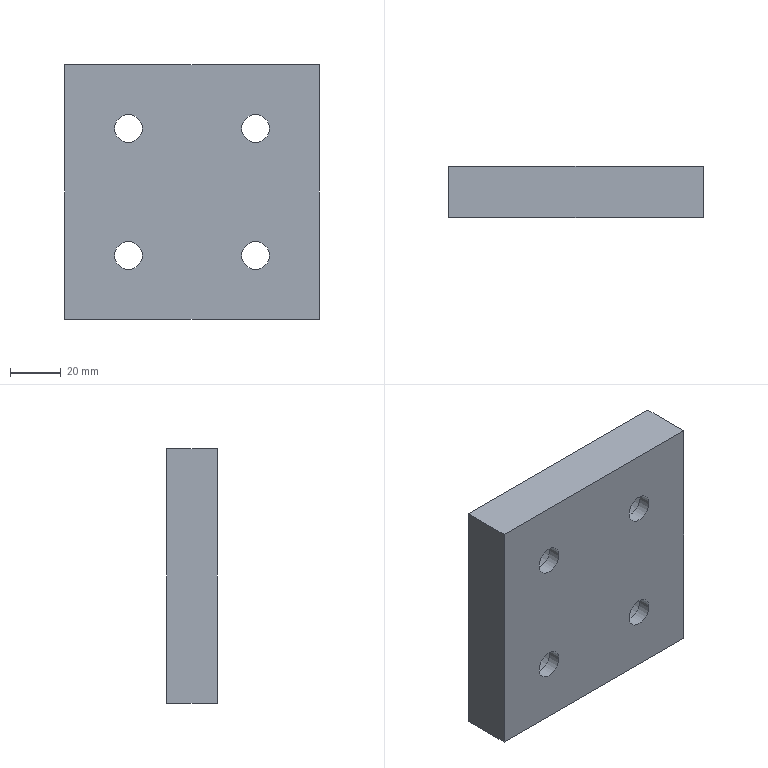Part | NX | features solid 2 | 1 solid | 18 faces | box 100 x 20 x 100 mm | volume 183668 mm3 | plane 10 | cylinder 8 | commonest cylinder face diameters 11 x4 17.5 x4
STEP:
#1=CARTESIAN_POINT('',(-1100.,530.,-135.));
#2=VERTEX_POINT('',#1);
#3=CARTESIAN_POINT('',(-1100.,510.,-135.));
#4=VERTEX_POINT('',#3);
#5=CARTESIAN_POINT('',(-1100.,520.,-135.));
#6=DIRECTION('',(0.,-1.,0.));
#7=VECTOR('',#6,1000.);
#8=LINE('',#5,#7);
#9=EDGE_CURVE('',#2,#4,#8,.T.);
#10=ORIENTED_EDGE('',*,*,#9,.F.);
#11=CARTESIAN_POINT('',(-1000.,530.,-135.));
#12=VERTEX_POINT('',#11);
#13=CARTESIAN_POINT('',(-1050.,530.,-135.));
#14=DIRECTION('',(-1.,0.,0.));
#15=VECTOR('',#14,1000.);
#16=LINE('',#13,#15);
#17=EDGE_CURVE('',#12,#2,#16,.T.);
#18=ORIENTED_EDGE('',*,*,#17,.F.);
#19=CARTESIAN_POINT('',(-1000.,510.,-135.));
#20=VERTEX_POINT('',#19);
#21=CARTESIAN_POINT('',(-1000.,520.,-135.));
#22=DIRECTION('',(0.,1.,0.));
#23=VECTOR('',#22,1000.);
#24=LINE('',#21,#23);
#25=EDGE_CURVE('',#20,#12,#24,.T.);
#26=ORIENTED_EDGE('',*,*,#25,.F.);
#27=CARTESIAN_POINT('',(-1050.,510.,-135.));
#28=DIRECTION('',(1.,0.,0.));
#29=VECTOR('',#28,1000.);
#30=LINE('',#27,#29);
#31=EDGE_CURVE('',#4,#20,#30,.T.);
#32=ORIENTED_EDGE('',*,*,#31,.F.);
#33=EDGE_LOOP('',(#10,#18,#26,#32));
#34=FACE_BOUND('',#33,.T.);
#35=CARTESIAN_POINT('',(-1050.,520.,-135.));
#36=DIRECTION('',(0.,0.,-1.));
#37=DIRECTION('',(0.,1.,0.));
#38=AXIS2_PLACEMENT_3D('',#35,#36,#37);
#39=PLANE('',#38);
#40=ADVANCED_FACE('',(#34),#39,.T.);
#41=CARTESIAN_POINT('',(-1100.,530.,-35.));
#42=VERTEX_POINT('',#41);
#43=CARTESIAN_POINT('',(-1100.,530.,-35.));
#44=DIRECTION('',(0.,0.,-1.));
#45=VECTOR('',#44,1000.);
#46=LINE('',#43,#45);
#47=EDGE_CURVE('',#42,#2,#46,.T.);
#48=ORIENTED_EDGE('',*,*,#47,.T.);
#49=ORIENTED_EDGE('',*,*,#9,.T.);
#50=CARTESIAN_POINT('',(-1100.,510.,-35.));
#51=VERTEX_POINT('',#50);
#52=CARTESIAN_POINT('',(-1100.,510.,-35.));
#53=DIRECTION('',(0.,0.,-1.));
#54=VECTOR('',#53,1000.);
#55=LINE('',#52,#54);
#56=EDGE_CURVE('',#51,#4,#55,.T.);
#57=ORIENTED_EDGE('',*,*,#56,.F.);
#58=CARTESIAN_POINT('',(-1100.,520.,-35.));
#59=DIRECTION('',(0.,1.,0.));
#60=VECTOR('',#59,1000.);
#61=LINE('',#58,#60);
#62=EDGE_CURVE('',#51,#42,#61,.T.);
#63=ORIENTED_EDGE('',*,*,#62,.T.);
#64=EDGE_LOOP('',(#48,#49,#57,#63));
#65=FACE_BOUND('',#64,.T.);
#66=CARTESIAN_POINT('',(-1100.,520.,-35.));
#67=DIRECTION('',(-1.,0.,0.));
#68=DIRECTION('',(0.,0.,1.));
#69=AXIS2_PLACEMENT_3D('',#66,#67,#68);
#70=PLANE('',#69);
#71=ADVANCED_FACE('',(#65),#70,.T.);
#72=CARTESIAN_POINT('',(-1025.,510.,-54.5));
#73=VERTEX_POINT('',#72);
#74=CARTESIAN_POINT('',(-1025.,510.,-60.));
#75=DIRECTION('',(0.,1.,0.));
#76=DIRECTION('',(0.,0.,1.));
#77=AXIS2_PLACEMENT_3D('',#74,#75,#76);
#78=CIRCLE('',#77,5.5);
#79=EDGE_CURVE('',#73,#73,#78,.T.);
#80=ORIENTED_EDGE('',*,*,#79,.T.);
#81=EDGE_LOOP('',(#80));
#82=FACE_BOUND('',#81,.T.);
#83=CARTESIAN_POINT('',(-1025.,510.,-104.5));
#84=VERTEX_POINT('',#83);
#85=CARTESIAN_POINT('',(-1025.,510.,-110.));
#86=DIRECTION('',(0.,1.,0.));
#87=DIRECTION('',(0.,0.,1.));
#88=AXIS2_PLACEMENT_3D('',#85,#86,#87);
#89=CIRCLE('',#88,5.5);
#90=EDGE_CURVE('',#84,#84,#89,.T.);
#91=ORIENTED_EDGE('',*,*,#90,.T.);
#92=EDGE_LOOP('',(#91));
#93=FACE_BOUND('',#92,.T.);
#94=CARTESIAN_POINT('',(-1075.,510.,-54.5));
#95=VERTEX_POINT('',#94);
#96=CARTESIAN_POINT('',(-1075.,510.,-60.));
#97=DIRECTION('',(0.,1.,0.));
#98=DIRECTION('',(0.,0.,1.));
#99=AXIS2_PLACEMENT_3D('',#96,#97,#98);
#100=CIRCLE('',#99,5.5);
#101=EDGE_CURVE('',#95,#95,#100,.T.);
#102=ORIENTED_EDGE('',*,*,#101,.T.);
#103=EDGE_LOOP('',(#102));
#104=FACE_BOUND('',#103,.T.);
#105=CARTESIAN_POINT('',(-1075.,510.,-104.5));
#106=VERTEX_POINT('',#105);
#107=CARTESIAN_POINT('',(-1075.,510.,-110.));
#108=DIRECTION('',(0.,1.,0.));
#109=DIRECTION('',(0.,0.,1.));
#110=AXIS2_PLACEMENT_3D('',#107,#108,#109);
#111=CIRCLE('',#110,5.5);
#112=EDGE_CURVE('',#106,#106,#111,.T.);
#113=ORIENTED_EDGE('',*,*,#112,.T.);
#114=EDGE_LOOP('',(#113));
#115=FACE_BOUND('',#114,.T.);
#116=ORIENTED_EDGE('',*,*,#56,.T.);
#117=ORIENTED_EDGE('',*,*,#31,.T.);
#118=CARTESIAN_POINT('',(-1000.,510.,-35.));
#119=VERTEX_POINT('',#118);
#120=CARTESIAN_POINT('',(-1000.,510.,-35.));
#121=DIRECTION('',(0.,0.,-1.));
#122=VECTOR('',#121,1000.);
#123=LINE('',#120,#122);
#124=EDGE_CURVE('',#119,#20,#123,.T.);
#125=ORIENTED_EDGE('',*,*,#124,.F.);
#126=CARTESIAN_POINT('',(-1050.,510.,-35.));
#127=DIRECTION('',(-1.,0.,0.));
#128=VECTOR('',#127,1000.);
#129=LINE('',#126,#128);
#130=EDGE_CURVE('',#119,#51,#129,.T.);
#131=ORIENTED_EDGE('',*,*,#130,.T.);
#132=EDGE_LOOP('',(#116,#117,#125,#131));
#133=FACE_BOUND('',#132,.T.);
#134=CARTESIAN_POINT('',(-1050.,510.,-35.));
#135=DIRECTION('',(0.,-1.,0.));
#136=DIRECTION('',(0.,0.,-1.));
#137=AXIS2_PLACEMENT_3D('',#134,#135,#136);
#138=PLANE('',#137);
#139=ADVANCED_FACE('',(#82,#93,#104,#115,#133),#138,.T.);
#140=ORIENTED_EDGE('',*,*,#124,.T.);
#141=ORIENTED_EDGE('',*,*,#25,.T.);
#142=CARTESIAN_POINT('',(-1000.,530.,-35.));
#143=VERTEX_POINT('',#142);
#144=CARTESIAN_POINT('',(-1000.,530.,-35.));
#145=DIRECTION('',(0.,0.,-1.));
#146=VECTOR('',#145,1000.);
#147=LINE('',#144,#146);
#148=EDGE_CURVE('',#143,#12,#147,.T.);
#149=ORIENTED_EDGE('',*,*,#148,.F.);
#150=CARTESIAN_POINT('',(-1000.,520.,-35.));
#151=DIRECTION('',(0.,-1.,0.));
#152=VECTOR('',#151,1000.);
#153=LINE('',#150,#152);
#154=EDGE_CURVE('',#143,#119,#153,.T.);
#155=ORIENTED_EDGE('',*,*,#154,.T.);
#156=EDGE_LOOP('',(#140,#141,#149,#155));
#157=FACE_BOUND('',#156,.T.);
#158=CARTESIAN_POINT('',(-1000.,520.,-35.));
#159=DIRECTION('',(1.,0.,0.));
#160=DIRECTION('',(0.,0.,-1.));
#161=AXIS2_PLACEMENT_3D('',#158,#159,#160);
#162=PLANE('',#161);
#163=ADVANCED_FACE('',(#157),#162,.T.);
#164=CARTESIAN_POINT('',(-1050.,530.,-35.));
#165=DIRECTION('',(1.,0.,0.));
#166=VECTOR('',#165,1000.);
#167=LINE('',#164,#166);
#168=EDGE_CURVE('',#42,#143,#167,.T.);
#169=ORIENTED_EDGE('',*,*,#168,.F.);
#170=ORIENTED_EDGE('',*,*,#62,.F.);
#171=ORIENTED_EDGE('',*,*,#130,.F.);
#172=ORIENTED_EDGE('',*,*,#154,.F.);
#173=EDGE_LOOP('',(#169,#170,#171,#172));
#174=FACE_BOUND('',#173,.T.);
#175=CARTESIAN_POINT('',(-1050.,520.,-35.));
#176=DIRECTION('',(0.,0.,1.));
#177=DIRECTION('',(0.,-1.,0.));
#178=AXIS2_PLACEMENT_3D('',#175,#176,#177);
#179=PLANE('',#178);
#180=ADVANCED_FACE('',(#174),#179,.T.);
#181=CARTESIAN_POINT('',(-1025.,530.,-68.75));
#182=VERTEX_POINT('',#181);
#183=CARTESIAN_POINT('',(-1025.,530.,-60.));
#184=DIRECTION('',(0.,-1.,0.));
#185=DIRECTION('',(0.,0.,-1.));
#186=AXIS2_PLACEMENT_3D('',#183,#184,#185);
#187=CIRCLE('',#186,8.75);
#188=EDGE_CURVE('',#182,#182,#187,.T.);
#189=ORIENTED_EDGE('',*,*,#188,.T.);
#190=EDGE_LOOP('',(#189));
#191=FACE_BOUND('',#190,.T.);
#192=CARTESIAN_POINT('',(-1025.,530.,-118.75));
#193=VERTEX_POINT('',#192);
#194=CARTESIAN_POINT('',(-1025.,530.,-110.));
#195=DIRECTION('',(0.,-1.,0.));
#196=DIRECTION('',(0.,0.,-1.));
#197=AXIS2_PLACEMENT_3D('',#194,#195,#196);
#198=CIRCLE('',#197,8.75);
#199=EDGE_CURVE('',#193,#193,#198,.T.);
#200=ORIENTED_EDGE('',*,*,#199,.T.);
#201=EDGE_LOOP('',(#200));
#202=FACE_BOUND('',#201,.T.);
#203=CARTESIAN_POINT('',(-1075.,530.,-68.75));
#204=VERTEX_POINT('',#203);
#205=CARTESIAN_POINT('',(-1075.,530.,-60.));
#206=DIRECTION('',(0.,-1.,0.));
#207=DIRECTION('',(0.,0.,-1.));
#208=AXIS2_PLACEMENT_3D('',#205,#206,#207);
#209=CIRCLE('',#208,8.75);
#210=EDGE_CURVE('',#204,#204,#209,.T.);
#211=ORIENTED_EDGE('',*,*,#210,.T.);
#212=EDGE_LOOP('',(#211));
#213=FACE_BOUND('',#212,.T.);
#214=CARTESIAN_POINT('',(-1075.,530.,-118.75));
#215=VERTEX_POINT('',#214);
#216=CARTESIAN_POINT('',(-1075.,530.,-110.));
#217=DIRECTION('',(0.,-1.,0.));
#218=DIRECTION('',(0.,0.,-1.));
#219=AXIS2_PLACEMENT_3D('',#216,#217,#218);
#220=CIRCLE('',#219,8.75);
#221=EDGE_CURVE('',#215,#215,#220,.T.);
#222=ORIENTED_EDGE('',*,*,#221,.T.);
#223=EDGE_LOOP('',(#222));
#224=FACE_BOUND('',#223,.T.);
#225=ORIENTED_EDGE('',*,*,#168,.T.);
#226=ORIENTED_EDGE('',*,*,#148,.T.);
#227=ORIENTED_EDGE('',*,*,#17,.T.);
#228=ORIENTED_EDGE('',*,*,#47,.F.);
#229=EDGE_LOOP('',(#225,#226,#227,#228));
#230=FACE_BOUND('',#229,.T.);
#231=CARTESIAN_POINT('',(-1050.,530.,-35.));
#232=DIRECTION('',(0.,1.,0.));
#233=DIRECTION('',(0.,0.,1.));
#234=AXIS2_PLACEMENT_3D('',#231,#232,#233);
#235=PLANE('',#234);
#236=ADVANCED_FACE('',(#191,#202,#213,#224,#230),#235,.T.);
#237=CARTESIAN_POINT('',(-1075.,515.,-115.5));
#238=VERTEX_POINT('',#237);
#239=CARTESIAN_POINT('',(-1075.,515.,-110.));
#240=DIRECTION('',(0.,-1.,0.));
#241=DIRECTION('',(0.,0.,-1.));
#242=AXIS2_PLACEMENT_3D('',#239,#240,#241);
#243=CIRCLE('',#242,5.5);
#244=EDGE_CURVE('',#238,#238,#243,.F.);
#245=ORIENTED_EDGE('',*,*,#244,.T.);
#246=EDGE_LOOP('',(#245));
#247=FACE_BOUND('',#246,.T.);
#248=ORIENTED_EDGE('',*,*,#112,.F.);
#249=EDGE_LOOP('',(#248));
#250=FACE_BOUND('',#249,.T.);
#251=CARTESIAN_POINT('',(-1075.,510.,-110.));
#252=DIRECTION('',(0.,1.,0.));
#253=DIRECTION('',(0.,0.,1.));
#254=AXIS2_PLACEMENT_3D('',#251,#252,#253);
#255=CYLINDRICAL_SURFACE('',#254,5.5);
#256=ADVANCED_FACE('',(#247,#250),#255,.F.);
#257=CARTESIAN_POINT('',(-1075.,515.,-101.25));
#258=VERTEX_POINT('',#257);
#259=CARTESIAN_POINT('',(-1075.,515.,-110.));
#260=DIRECTION('',(0.,1.,0.));
#261=DIRECTION('',(0.,0.,1.));
#262=AXIS2_PLACEMENT_3D('',#259,#260,#261);
#263=CIRCLE('',#262,8.75);
#264=EDGE_CURVE('',#258,#258,#263,.T.);
#265=ORIENTED_EDGE('',*,*,#264,.T.);
#266=EDGE_LOOP('',(#265));
#267=FACE_BOUND('',#266,.T.);
#268=ORIENTED_EDGE('',*,*,#244,.F.);
#269=EDGE_LOOP('',(#268));
#270=FACE_BOUND('',#269,.T.);
#271=CARTESIAN_POINT('',(-1075.,515.,-110.));
#272=DIRECTION('',(0.,-1.,0.));
#273=DIRECTION('',(0.,0.,-1.));
#274=AXIS2_PLACEMENT_3D('',#271,#272,#273);
#275=PLANE('',#274);
#276=ADVANCED_FACE('',(#267,#270),#275,.F.);
#277=ORIENTED_EDGE('',*,*,#221,.F.);
#278=EDGE_LOOP('',(#277));
#279=FACE_BOUND('',#278,.T.);
#280=ORIENTED_EDGE('',*,*,#264,.F.);
#281=EDGE_LOOP('',(#280));
#282=FACE_BOUND('',#281,.T.);
#283=CARTESIAN_POINT('',(-1075.,515.,-110.));
#284=DIRECTION('',(0.,1.,0.));
#285=DIRECTION('',(0.,0.,1.));
#286=AXIS2_PLACEMENT_3D('',#283,#284,#285);
#287=CYLINDRICAL_SURFACE('',#286,8.75);
#288=ADVANCED_FACE('',(#279,#282),#287,.F.);
#289=CARTESIAN_POINT('',(-1075.,515.,-65.5));
#290=VERTEX_POINT('',#289);
#291=CARTESIAN_POINT('',(-1075.,515.,-60.));
#292=DIRECTION('',(0.,-1.,0.));
#293=DIRECTION('',(0.,0.,-1.));
#294=AXIS2_PLACEMENT_3D('',#291,#292,#293);
#295=CIRCLE('',#294,5.5);
#296=EDGE_CURVE('',#290,#290,#295,.F.);
#297=ORIENTED_EDGE('',*,*,#296,.T.);
#298=EDGE_LOOP('',(#297));
#299=FACE_BOUND('',#298,.T.);
#300=ORIENTED_EDGE('',*,*,#101,.F.);
#301=EDGE_LOOP('',(#300));
#302=FACE_BOUND('',#301,.T.);
#303=CARTESIAN_POINT('',(-1075.,510.,-60.));
#304=DIRECTION('',(0.,1.,0.));
#305=DIRECTION('',(0.,0.,1.));
#306=AXIS2_PLACEMENT_3D('',#303,#304,#305);
#307=CYLINDRICAL_SURFACE('',#306,5.5);
#308=ADVANCED_FACE('',(#299,#302),#307,.F.);
#309=CARTESIAN_POINT('',(-1075.,515.,-51.25));
#310=VERTEX_POINT('',#309);
#311=CARTESIAN_POINT('',(-1075.,515.,-60.));
#312=DIRECTION('',(0.,1.,0.));
#313=DIRECTION('',(0.,0.,1.));
#314=AXIS2_PLACEMENT_3D('',#311,#312,#313);
#315=CIRCLE('',#314,8.75);
#316=EDGE_CURVE('',#310,#310,#315,.T.);
#317=ORIENTED_EDGE('',*,*,#316,.T.);
#318=EDGE_LOOP('',(#317));
#319=FACE_BOUND('',#318,.T.);
#320=ORIENTED_EDGE('',*,*,#296,.F.);
#321=EDGE_LOOP('',(#320));
#322=FACE_BOUND('',#321,.T.);
#323=CARTESIAN_POINT('',(-1075.,515.,-60.));
#324=DIRECTION('',(0.,-1.,0.));
#325=DIRECTION('',(0.,0.,-1.));
#326=AXIS2_PLACEMENT_3D('',#323,#324,#325);
#327=PLANE('',#326);
#328=ADVANCED_FACE('',(#319,#322),#327,.F.);
#329=ORIENTED_EDGE('',*,*,#210,.F.);
#330=EDGE_LOOP('',(#329));
#331=FACE_BOUND('',#330,.T.);
#332=ORIENTED_EDGE('',*,*,#316,.F.);
#333=EDGE_LOOP('',(#332));
#334=FACE_BOUND('',#333,.T.);
#335=CARTESIAN_POINT('',(-1075.,515.,-60.));
#336=DIRECTION('',(0.,1.,0.));
#337=DIRECTION('',(0.,0.,1.));
#338=AXIS2_PLACEMENT_3D('',#335,#336,#337);
#339=CYLINDRICAL_SURFACE('',#338,8.75);
#340=ADVANCED_FACE('',(#331,#334),#339,.F.);
#341=CARTESIAN_POINT('',(-1025.,515.,-115.5));
#342=VERTEX_POINT('',#341);
#343=CARTESIAN_POINT('',(-1025.,515.,-110.));
#344=DIRECTION('',(0.,-1.,0.));
#345=DIRECTION('',(0.,0.,-1.));
#346=AXIS2_PLACEMENT_3D('',#343,#344,#345);
#347=CIRCLE('',#346,5.5);
#348=EDGE_CURVE('',#342,#342,#347,.F.);
#349=ORIENTED_EDGE('',*,*,#348,.T.);
#350=EDGE_LOOP('',(#349));
#351=FACE_BOUND('',#350,.T.);
#352=ORIENTED_EDGE('',*,*,#90,.F.);
#353=EDGE_LOOP('',(#352));
#354=FACE_BOUND('',#353,.T.);
#355=CARTESIAN_POINT('',(-1025.,510.,-110.));
#356=DIRECTION('',(0.,1.,0.));
#357=DIRECTION('',(0.,0.,1.));
#358=AXIS2_PLACEMENT_3D('',#355,#356,#357);
#359=CYLINDRICAL_SURFACE('',#358,5.5);
#360=ADVANCED_FACE('',(#351,#354),#359,.F.);
#361=CARTESIAN_POINT('',(-1025.,515.,-101.25));
#362=VERTEX_POINT('',#361);
#363=CARTESIAN_POINT('',(-1025.,515.,-110.));
#364=DIRECTION('',(0.,1.,0.));
#365=DIRECTION('',(0.,0.,1.));
#366=AXIS2_PLACEMENT_3D('',#363,#364,#365);
#367=CIRCLE('',#366,8.75);
#368=EDGE_CURVE('',#362,#362,#367,.T.);
#369=ORIENTED_EDGE('',*,*,#368,.T.);
#370=EDGE_LOOP('',(#369));
#371=FACE_BOUND('',#370,.T.);
#372=ORIENTED_EDGE('',*,*,#348,.F.);
#373=EDGE_LOOP('',(#372));
#374=FACE_BOUND('',#373,.T.);
#375=CARTESIAN_POINT('',(-1025.,515.,-110.));
#376=DIRECTION('',(0.,-1.,0.));
#377=DIRECTION('',(0.,0.,-1.));
#378=AXIS2_PLACEMENT_3D('',#375,#376,#377);
#379=PLANE('',#378);
#380=ADVANCED_FACE('',(#371,#374),#379,.F.);
#381=ORIENTED_EDGE('',*,*,#199,.F.);
#382=EDGE_LOOP('',(#381));
#383=FACE_BOUND('',#382,.T.);
#384=ORIENTED_EDGE('',*,*,#368,.F.);
#385=EDGE_LOOP('',(#384));
#386=FACE_BOUND('',#385,.T.);
#387=CARTESIAN_POINT('',(-1025.,515.,-110.));
#388=DIRECTION('',(0.,1.,0.));
#389=DIRECTION('',(0.,0.,1.));
#390=AXIS2_PLACEMENT_3D('',#387,#388,#389);
#391=CYLINDRICAL_SURFACE('',#390,8.75);
#392=ADVANCED_FACE('',(#383,#386),#391,.F.);
#393=CARTESIAN_POINT('',(-1025.,515.,-65.5));
#394=VERTEX_POINT('',#393);
#395=CARTESIAN_POINT('',(-1025.,515.,-60.));
#396=DIRECTION('',(0.,-1.,0.));
#397=DIRECTION('',(0.,0.,-1.));
#398=AXIS2_PLACEMENT_3D('',#395,#396,#397);
#399=CIRCLE('',#398,5.5);
#400=EDGE_CURVE('',#394,#394,#399,.F.);
#401=ORIENTED_EDGE('',*,*,#400,.T.);
#402=EDGE_LOOP('',(#401));
#403=FACE_BOUND('',#402,.T.);
#404=ORIENTED_EDGE('',*,*,#79,.F.);
#405=EDGE_LOOP('',(#404));
#406=FACE_BOUND('',#405,.T.);
#407=CARTESIAN_POINT('',(-1025.,510.,-60.));
#408=DIRECTION('',(0.,1.,0.));
#409=DIRECTION('',(0.,0.,1.));
#410=AXIS2_PLACEMENT_3D('',#407,#408,#409);
#411=CYLINDRICAL_SURFACE('',#410,5.5);
#412=ADVANCED_FACE('',(#403,#406),#411,.F.);
#413=CARTESIAN_POINT('',(-1025.,515.,-51.25));
#414=VERTEX_POINT('',#413);
#415=CARTESIAN_POINT('',(-1025.,515.,-60.));
#416=DIRECTION('',(0.,1.,0.));
#417=DIRECTION('',(0.,0.,1.));
#418=AXIS2_PLACEMENT_3D('',#415,#416,#417);
#419=CIRCLE('',#418,8.75);
#420=EDGE_CURVE('',#414,#414,#419,.T.);
#421=ORIENTED_EDGE('',*,*,#420,.T.);
#422=EDGE_LOOP('',(#421));
#423=FACE_BOUND('',#422,.T.);
#424=ORIENTED_EDGE('',*,*,#400,.F.);
#425=EDGE_LOOP('',(#424));
#426=FACE_BOUND('',#425,.T.);
#427=CARTESIAN_POINT('',(-1025.,515.,-60.));
#428=DIRECTION('',(0.,-1.,0.));
#429=DIRECTION('',(0.,0.,-1.));
#430=AXIS2_PLACEMENT_3D('',#427,#428,#429);
#431=PLANE('',#430);
#432=ADVANCED_FACE('',(#423,#426),#431,.F.);
#433=ORIENTED_EDGE('',*,*,#188,.F.);
#434=EDGE_LOOP('',(#433));
#435=FACE_BOUND('',#434,.T.);
#436=ORIENTED_EDGE('',*,*,#420,.F.);
#437=EDGE_LOOP('',(#436));
#438=FACE_BOUND('',#437,.T.);
#439=CARTESIAN_POINT('',(-1025.,515.,-60.));
#440=DIRECTION('',(0.,1.,0.));
#441=DIRECTION('',(0.,0.,1.));
#442=AXIS2_PLACEMENT_3D('',#439,#440,#441);
#443=CYLINDRICAL_SURFACE('',#442,8.75);
#444=ADVANCED_FACE('',(#435,#438),#443,.F.);
#445=CLOSED_SHELL('',(#40,#71,#139,#163,#180,#236,#256,#276,#288,#308,#328,#340,#360,#380,#392,#412,#432,#444));
#446=MANIFOLD_SOLID_BREP('',#445);
#447=(LENGTH_UNIT()NAMED_UNIT(*)SI_UNIT(.MILLI.,.METRE.));
#448=UNCERTAINTY_MEASURE_WITH_UNIT(LENGTH_MEASURE(0.00001),#447,'','');
#449=(NAMED_UNIT(*)PLANE_ANGLE_UNIT()SI_UNIT($,.RADIAN.));
#450=(NAMED_UNIT(*)SI_UNIT($,.STERADIAN.)SOLID_ANGLE_UNIT());
#451=(GEOMETRIC_REPRESENTATION_CONTEXT(3)GLOBAL_UNCERTAINTY_ASSIGNED_CONTEXT((#448))GLOBAL_UNIT_ASSIGNED_CONTEXT((#447,#449,#450))REPRESENTATION_CONTEXT('',''));
#452=ADVANCED_BREP_SHAPE_REPRESENTATION('',(#446),#451);